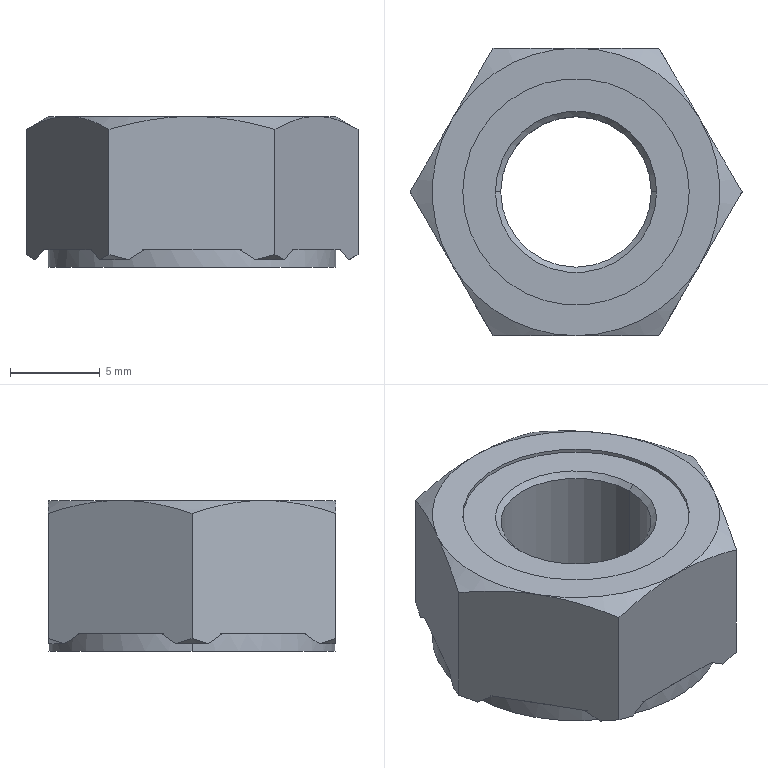Part | STEP file | SOLID | 1 solid | 43 faces | box 18.475 x 16 x 8.4 mm | volume 1358 mm3 | cone 22 | plane 15 | cylinder 6 | commonest cylinder face diameters 8.376 x2 12.6 x2 16 x2